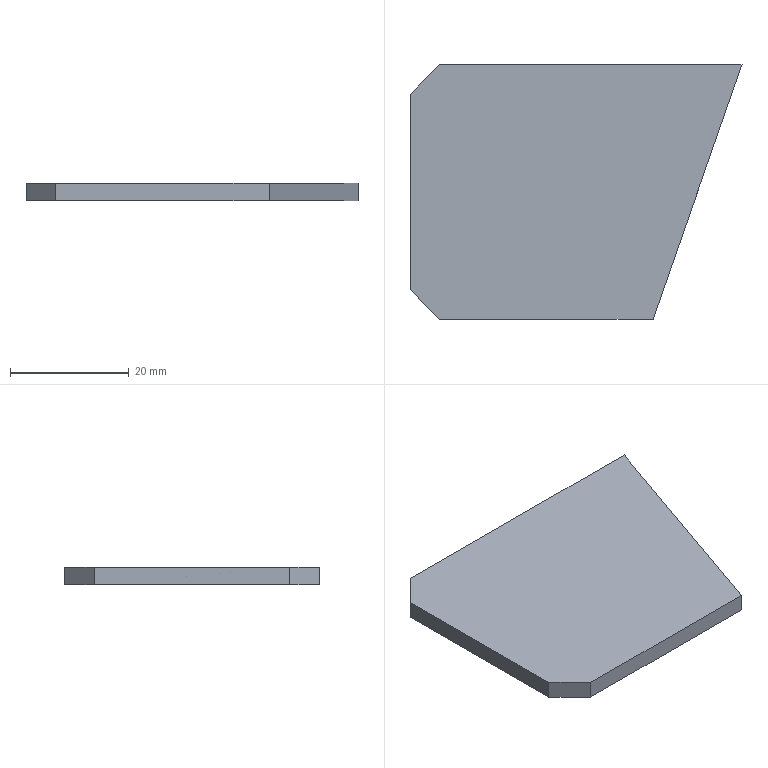Part | 1 solid | 8 faces | box 56 x 43 x 3 mm | volume 6182 mm3 | plane 8
STEP:
#1=CARTESIAN_POINT('',(56.,21.5,-3.));
#2=VERTEX_POINT('',#1);
#3=CARTESIAN_POINT('',(5.,21.5,-3.));
#4=VERTEX_POINT('',#3);
#5=CARTESIAN_POINT('',(56.,21.5,-3.));
#6=DIRECTION('',(-1.,0.,0.));
#7=VECTOR('',#6,1000.);
#8=LINE('',#5,#7);
#9=EDGE_CURVE('',#2,#4,#8,.T.);
#10=ORIENTED_EDGE('',*,*,#9,.T.);
#11=CARTESIAN_POINT('',(5.,21.5,0.));
#12=VERTEX_POINT('',#11);
#13=CARTESIAN_POINT('',(5.,21.5,-3.));
#14=DIRECTION('',(0.,0.,1.));
#15=VECTOR('',#14,1000.);
#16=LINE('',#13,#15);
#17=EDGE_CURVE('',#4,#12,#16,.T.);
#18=ORIENTED_EDGE('',*,*,#17,.T.);
#19=CARTESIAN_POINT('',(56.,21.5,0.));
#20=VERTEX_POINT('',#19);
#21=CARTESIAN_POINT('',(56.,21.5,0.));
#22=DIRECTION('',(-1.,0.,0.));
#23=VECTOR('',#22,1000.);
#24=LINE('',#21,#23);
#25=EDGE_CURVE('',#20,#12,#24,.T.);
#26=ORIENTED_EDGE('',*,*,#25,.F.);
#27=CARTESIAN_POINT('',(56.,21.5,-3.));
#28=DIRECTION('',(0.,0.,1.));
#29=VECTOR('',#28,1000.);
#30=LINE('',#27,#29);
#31=EDGE_CURVE('',#2,#20,#30,.T.);
#32=ORIENTED_EDGE('',*,*,#31,.F.);
#33=EDGE_LOOP('',(#10,#18,#26,#32));
#34=FACE_OUTER_BOUND('',#33,.T.);
#35=CARTESIAN_POINT('',(56.,21.5,-3.));
#36=DIRECTION('',(0.,1.,0.));
#37=DIRECTION('',(-1.,0.,0.));
#38=AXIS2_PLACEMENT_3D('',#35,#36,#37);
#39=PLANE('',#38);
#40=ADVANCED_FACE('',(#34),#39,.T.);
#41=CARTESIAN_POINT('',(41.,-21.5,0.));
#42=VERTEX_POINT('',#41);
#43=CARTESIAN_POINT('',(41.,-21.5,0.));
#44=DIRECTION('',(0.3294,0.9442,0.));
#45=VECTOR('',#44,1000.);
#46=LINE('',#43,#45);
#47=EDGE_CURVE('',#42,#20,#46,.T.);
#48=ORIENTED_EDGE('',*,*,#47,.F.);
#49=CARTESIAN_POINT('',(41.,-21.5,-3.));
#50=VERTEX_POINT('',#49);
#51=CARTESIAN_POINT('',(41.,-21.5,-3.));
#52=DIRECTION('',(0.,0.,1.));
#53=VECTOR('',#52,1000.);
#54=LINE('',#51,#53);
#55=EDGE_CURVE('',#50,#42,#54,.T.);
#56=ORIENTED_EDGE('',*,*,#55,.F.);
#57=CARTESIAN_POINT('',(41.,-21.5,-3.));
#58=DIRECTION('',(0.3294,0.9442,0.));
#59=VECTOR('',#58,1000.);
#60=LINE('',#57,#59);
#61=EDGE_CURVE('',#50,#2,#60,.T.);
#62=ORIENTED_EDGE('',*,*,#61,.T.);
#63=ORIENTED_EDGE('',*,*,#31,.T.);
#64=EDGE_LOOP('',(#48,#56,#62,#63));
#65=FACE_OUTER_BOUND('',#64,.T.);
#66=CARTESIAN_POINT('',(41.,-21.5,-3.));
#67=DIRECTION('',(0.9442,-0.3294,0.));
#68=DIRECTION('',(0.3294,0.9442,0.));
#69=AXIS2_PLACEMENT_3D('',#66,#67,#68);
#70=PLANE('',#69);
#71=ADVANCED_FACE('',(#65),#70,.T.);
#72=CARTESIAN_POINT('',(5.,-21.5,0.));
#73=VERTEX_POINT('',#72);
#74=CARTESIAN_POINT('',(0.,-21.5,0.));
#75=DIRECTION('',(1.,0.,0.));
#76=VECTOR('',#75,1000.);
#77=LINE('',#74,#76);
#78=EDGE_CURVE('',#73,#42,#77,.T.);
#79=ORIENTED_EDGE('',*,*,#78,.F.);
#80=CARTESIAN_POINT('',(5.,-21.5,-3.));
#81=VERTEX_POINT('',#80);
#82=CARTESIAN_POINT('',(5.,-21.5,-3.));
#83=DIRECTION('',(0.,0.,-1.));
#84=VECTOR('',#83,1000.);
#85=LINE('',#82,#84);
#86=EDGE_CURVE('',#73,#81,#85,.T.);
#87=ORIENTED_EDGE('',*,*,#86,.T.);
#88=CARTESIAN_POINT('',(0.,-21.5,-3.));
#89=DIRECTION('',(1.,0.,0.));
#90=VECTOR('',#89,1000.);
#91=LINE('',#88,#90);
#92=EDGE_CURVE('',#81,#50,#91,.T.);
#93=ORIENTED_EDGE('',*,*,#92,.T.);
#94=ORIENTED_EDGE('',*,*,#55,.T.);
#95=EDGE_LOOP('',(#79,#87,#93,#94));
#96=FACE_OUTER_BOUND('',#95,.T.);
#97=CARTESIAN_POINT('',(0.,-21.5,-3.));
#98=DIRECTION('',(0.,-1.,0.));
#99=DIRECTION('',(0.,0.,-1.));
#100=AXIS2_PLACEMENT_3D('',#97,#98,#99);
#101=PLANE('',#100);
#102=ADVANCED_FACE('',(#96),#101,.T.);
#103=CARTESIAN_POINT('',(0.,16.5,-3.));
#104=VERTEX_POINT('',#103);
#105=CARTESIAN_POINT('',(0.,-16.5,-3.));
#106=VERTEX_POINT('',#105);
#107=CARTESIAN_POINT('',(0.,21.5,-3.));
#108=DIRECTION('',(0.,-1.,0.));
#109=VECTOR('',#108,1000.);
#110=LINE('',#107,#109);
#111=EDGE_CURVE('',#104,#106,#110,.T.);
#112=ORIENTED_EDGE('',*,*,#111,.T.);
#113=CARTESIAN_POINT('',(0.,-16.5,0.));
#114=VERTEX_POINT('',#113);
#115=CARTESIAN_POINT('',(0.,-16.5,-3.));
#116=DIRECTION('',(0.,0.,1.));
#117=VECTOR('',#116,1000.);
#118=LINE('',#115,#117);
#119=EDGE_CURVE('',#106,#114,#118,.T.);
#120=ORIENTED_EDGE('',*,*,#119,.T.);
#121=CARTESIAN_POINT('',(0.,16.5,0.));
#122=VERTEX_POINT('',#121);
#123=CARTESIAN_POINT('',(0.,21.5,0.));
#124=DIRECTION('',(0.,-1.,0.));
#125=VECTOR('',#124,1000.);
#126=LINE('',#123,#125);
#127=EDGE_CURVE('',#122,#114,#126,.T.);
#128=ORIENTED_EDGE('',*,*,#127,.F.);
#129=CARTESIAN_POINT('',(0.,16.5,-3.));
#130=DIRECTION('',(0.,0.,-1.));
#131=VECTOR('',#130,1000.);
#132=LINE('',#129,#131);
#133=EDGE_CURVE('',#122,#104,#132,.T.);
#134=ORIENTED_EDGE('',*,*,#133,.T.);
#135=EDGE_LOOP('',(#112,#120,#128,#134));
#136=FACE_OUTER_BOUND('',#135,.T.);
#137=CARTESIAN_POINT('',(0.,21.5,-3.));
#138=DIRECTION('',(-1.,0.,0.));
#139=DIRECTION('',(0.,-1.,0.));
#140=AXIS2_PLACEMENT_3D('',#137,#138,#139);
#141=PLANE('',#140);
#142=ADVANCED_FACE('',(#136),#141,.T.);
#143=ORIENTED_EDGE('',*,*,#92,.F.);
#144=CARTESIAN_POINT('',(0.,-16.5,-3.));
#145=DIRECTION('',(-0.7071,0.7071,0.));
#146=VECTOR('',#145,1000.);
#147=LINE('',#144,#146);
#148=EDGE_CURVE('',#81,#106,#147,.T.);
#149=ORIENTED_EDGE('',*,*,#148,.T.);
#150=ORIENTED_EDGE('',*,*,#111,.F.);
#151=CARTESIAN_POINT('',(5.,21.5,-3.));
#152=DIRECTION('',(0.7071,0.7071,0.));
#153=VECTOR('',#152,1000.);
#154=LINE('',#151,#153);
#155=EDGE_CURVE('',#104,#4,#154,.T.);
#156=ORIENTED_EDGE('',*,*,#155,.T.);
#157=ORIENTED_EDGE('',*,*,#9,.F.);
#158=ORIENTED_EDGE('',*,*,#61,.F.);
#159=EDGE_LOOP('',(#143,#149,#150,#156,#157,#158));
#160=FACE_OUTER_BOUND('',#159,.T.);
#161=CARTESIAN_POINT('',(0.,0.,-3.));
#162=DIRECTION('',(0.,0.,1.));
#163=DIRECTION('',(1.,0.,0.));
#164=AXIS2_PLACEMENT_3D('',#161,#162,#163);
#165=PLANE('',#164);
#166=ADVANCED_FACE('',(#160),#165,.F.);
#167=ORIENTED_EDGE('',*,*,#127,.T.);
#168=CARTESIAN_POINT('',(-8.25,-8.25,0.));
#169=DIRECTION('',(0.7071,-0.7071,0.));
#170=VECTOR('',#169,1000.);
#171=LINE('',#168,#170);
#172=EDGE_CURVE('',#114,#73,#171,.T.);
#173=ORIENTED_EDGE('',*,*,#172,.T.);
#174=ORIENTED_EDGE('',*,*,#78,.T.);
#175=ORIENTED_EDGE('',*,*,#47,.T.);
#176=ORIENTED_EDGE('',*,*,#25,.T.);
#177=CARTESIAN_POINT('',(-8.25,8.25,0.));
#178=DIRECTION('',(-0.7071,-0.7071,0.));
#179=VECTOR('',#178,1000.);
#180=LINE('',#177,#179);
#181=EDGE_CURVE('',#12,#122,#180,.T.);
#182=ORIENTED_EDGE('',*,*,#181,.T.);
#183=EDGE_LOOP('',(#167,#173,#174,#175,#176,#182));
#184=FACE_OUTER_BOUND('',#183,.T.);
#185=CARTESIAN_POINT('',(0.,0.,0.));
#186=DIRECTION('',(0.,0.,1.));
#187=DIRECTION('',(1.,0.,0.));
#188=AXIS2_PLACEMENT_3D('',#185,#186,#187);
#189=PLANE('',#188);
#190=ADVANCED_FACE('',(#184),#189,.T.);
#191=ORIENTED_EDGE('',*,*,#148,.F.);
#192=ORIENTED_EDGE('',*,*,#86,.F.);
#193=ORIENTED_EDGE('',*,*,#172,.F.);
#194=ORIENTED_EDGE('',*,*,#119,.F.);
#195=EDGE_LOOP('',(#191,#192,#193,#194));
#196=FACE_OUTER_BOUND('',#195,.T.);
#197=CARTESIAN_POINT('',(0.,-16.5,-3.));
#198=DIRECTION('',(0.7071,0.7071,0.));
#199=DIRECTION('',(0.,0.,1.));
#200=AXIS2_PLACEMENT_3D('',#197,#198,#199);
#201=PLANE('',#200);
#202=ADVANCED_FACE('',(#196),#201,.F.);
#203=ORIENTED_EDGE('',*,*,#155,.F.);
#204=ORIENTED_EDGE('',*,*,#133,.F.);
#205=ORIENTED_EDGE('',*,*,#181,.F.);
#206=ORIENTED_EDGE('',*,*,#17,.F.);
#207=EDGE_LOOP('',(#203,#204,#205,#206));
#208=FACE_OUTER_BOUND('',#207,.T.);
#209=CARTESIAN_POINT('',(5.,21.5,-3.));
#210=DIRECTION('',(0.7071,-0.7071,0.));
#211=DIRECTION('',(0.,0.,1.));
#212=AXIS2_PLACEMENT_3D('',#209,#210,#211);
#213=PLANE('',#212);
#214=ADVANCED_FACE('',(#208),#213,.F.);
#215=CLOSED_SHELL('',(#40,#71,#102,#142,#166,#190,#202,#214));
#216=MANIFOLD_SOLID_BREP('',#215);
#217=CARTESIAN_POINT('',(0.,0.,0.));
#218=DIRECTION('',(0.,0.,1.));
#219=DIRECTION('',(1.,0.,0.));
#220=AXIS2_PLACEMENT_3D('',#217,#218,#219);
#221=(LENGTH_UNIT()NAMED_UNIT(*)SI_UNIT(.MILLI.,.METRE.));
#222=UNCERTAINTY_MEASURE_WITH_UNIT(LENGTH_MEASURE(0.00001),#221,'','');
#223=(NAMED_UNIT(*)PLANE_ANGLE_UNIT()SI_UNIT($,.RADIAN.));
#224=(NAMED_UNIT(*)SI_UNIT($,.STERADIAN.)SOLID_ANGLE_UNIT());
#225=(GEOMETRIC_REPRESENTATION_CONTEXT(3)GLOBAL_UNCERTAINTY_ASSIGNED_CONTEXT((#222))GLOBAL_UNIT_ASSIGNED_CONTEXT((#221,#223,#224))REPRESENTATION_CONTEXT('',''));
#226=ADVANCED_BREP_SHAPE_REPRESENTATION('',(#216,#220),#225);